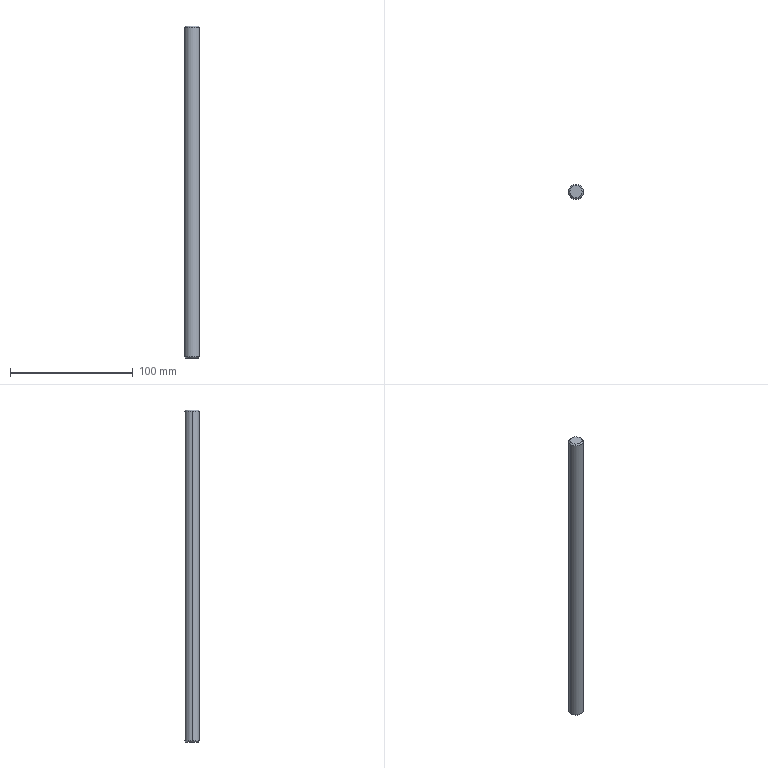Part | STEP file | BPSP-11-11 12Chrome Rod_Default | 1 solid | 12 faces | box 12 x 12 x 270 mm | volume 30254 mm3 | cone 6 | cylinder 4 | plane 2 | commonest cylinder face diameters 4.2 x2 12 x2
STEP:
#1=CARTESIAN_POINT('',(0.,0.,0.));
#2=DIRECTION('',(0.,0.,1.));
#3=DIRECTION('',(1.,0.,0.));
#4=AXIS2_PLACEMENT_3D('',#1,#2,#3);
#5=CARTESIAN_POINT('',(-2.1,0.,17.4));
#6=VERTEX_POINT('',#5);
#7=CARTESIAN_POINT('',(-2.1,0.,0.));
#8=VERTEX_POINT('',#7);
#9=CARTESIAN_POINT('',(-2.1,0.,0.));
#10=DIRECTION('',(0.,0.,-1.));
#11=VECTOR('',#10,1.);
#12=LINE('',#9,#11);
#13=CARTESIAN_POINT('',(0.,0.,0.));
#14=DIRECTION('',(0.,0.,-1.));
#15=DIRECTION('',(-1.,0.,0.));
#16=AXIS2_PLACEMENT_3D('',#13,#14,#15);
#17=CYLINDRICAL_SURFACE('',#16,2.1);
#18=CARTESIAN_POINT('',(6.283,0.));
#19=DIRECTION('',(0.,1.));
#20=VECTOR('',#19,1.);
#21=LINE('',#18,#20);
#22=(GEOMETRIC_REPRESENTATION_CONTEXT(2)PARAMETRIC_REPRESENTATION_CONTEXT()REPRESENTATION_CONTEXT('',''));
#23=DEFINITIONAL_REPRESENTATION('',(#21),#22);
#24=PCURVE('',#17,#23);
#25=CARTESIAN_POINT('',(0.,0.,0.));
#26=DIRECTION('',(0.,0.,-1.));
#27=DIRECTION('',(-1.,0.,0.));
#28=AXIS2_PLACEMENT_3D('',#25,#26,#27);
#29=CYLINDRICAL_SURFACE('',#28,2.1);
#30=CARTESIAN_POINT('',(0.,0.));
#31=DIRECTION('',(0.,1.));
#32=VECTOR('',#31,1.);
#33=LINE('',#30,#32);
#34=(GEOMETRIC_REPRESENTATION_CONTEXT(2)PARAMETRIC_REPRESENTATION_CONTEXT()REPRESENTATION_CONTEXT('',''));
#35=DEFINITIONAL_REPRESENTATION('',(#33),#34);
#36=PCURVE('',#29,#35);
#37=SURFACE_CURVE('',#12,(#24,#36),.PCURVE_S1.);
#38=EDGE_CURVE('',#6,#8,#37,.T.);
#39=ORIENTED_EDGE('',*,*,#38,.T.);
#40=CARTESIAN_POINT('',(2.1,0.,0.));
#41=VERTEX_POINT('',#40);
#42=CARTESIAN_POINT('',(0.,0.,0.));
#43=DIRECTION('',(0.,0.,-1.));
#44=DIRECTION('',(-1.,0.,0.));
#45=AXIS2_PLACEMENT_3D('',#42,#43,#44);
#46=CIRCLE('',#45,2.1);
#47=CARTESIAN_POINT('',(0.,0.));
#48=DIRECTION('',(1.,0.));
#49=VECTOR('',#48,1.);
#50=LINE('',#47,#49);
#51=(GEOMETRIC_REPRESENTATION_CONTEXT(2)PARAMETRIC_REPRESENTATION_CONTEXT()REPRESENTATION_CONTEXT('',''));
#52=DEFINITIONAL_REPRESENTATION('',(#50),#51);
#53=PCURVE('',#17,#52);
#54=CARTESIAN_POINT('',(0.,0.,0.));
#55=DIRECTION('',(0.,0.,1.));
#56=DIRECTION('',(1.,0.,0.));
#57=AXIS2_PLACEMENT_3D('',#54,#55,#56);
#58=PLANE('',#57);
#59=CARTESIAN_POINT('',(-2.1,0.));
#60=CARTESIAN_POINT('',(-2.1,3.637));
#61=CARTESIAN_POINT('',(1.05,1.819));
#62=CARTESIAN_POINT('',(4.2,0.));
#63=CARTESIAN_POINT('',(1.05,-1.819));
#64=CARTESIAN_POINT('',(-2.1,-3.637));
#65=CARTESIAN_POINT('',(-2.1,0.));
#66=(BOUNDED_CURVE()B_SPLINE_CURVE(2,(#59,#60,#61,#62,#63,#64,#65),.UNSPECIFIED.,.T.,.F.)B_SPLINE_CURVE_WITH_KNOTS((1,2,2,2,2,1),(-2.094,0.,2.094,4.189,6.283,8.378),.UNSPECIFIED.)CURVE()GEOMETRIC_REPRESENTATION_ITEM()RATIONAL_B_SPLINE_CURVE((1.,0.5,1.,0.5,1.,0.5,1.))REPRESENTATION_ITEM(''));
#67=(GEOMETRIC_REPRESENTATION_CONTEXT(2)PARAMETRIC_REPRESENTATION_CONTEXT()REPRESENTATION_CONTEXT('',''));
#68=DEFINITIONAL_REPRESENTATION('',(#66),#67);
#69=PCURVE('',#58,#68);
#70=SURFACE_CURVE('',#46,(#53,#69),.PCURVE_S1.);
#71=EDGE_CURVE('',#41,#8,#70,.T.);
#72=ORIENTED_EDGE('',*,*,#71,.F.);
#73=CARTESIAN_POINT('',(2.1,0.,17.4));
#74=VERTEX_POINT('',#73);
#75=CARTESIAN_POINT('',(2.1,0.,0.));
#76=DIRECTION('',(0.,0.,-1.));
#77=VECTOR('',#76,1.);
#78=LINE('',#75,#77);
#79=CARTESIAN_POINT('',(3.142,0.));
#80=DIRECTION('',(0.,1.));
#81=VECTOR('',#80,1.);
#82=LINE('',#79,#81);
#83=(GEOMETRIC_REPRESENTATION_CONTEXT(2)PARAMETRIC_REPRESENTATION_CONTEXT()REPRESENTATION_CONTEXT('',''));
#84=DEFINITIONAL_REPRESENTATION('',(#82),#83);
#85=PCURVE('',#17,#84);
#86=CARTESIAN_POINT('',(3.142,0.));
#87=DIRECTION('',(0.,1.));
#88=VECTOR('',#87,1.);
#89=LINE('',#86,#88);
#90=(GEOMETRIC_REPRESENTATION_CONTEXT(2)PARAMETRIC_REPRESENTATION_CONTEXT()REPRESENTATION_CONTEXT('',''));
#91=DEFINITIONAL_REPRESENTATION('',(#89),#90);
#92=PCURVE('',#29,#91);
#93=SURFACE_CURVE('',#78,(#85,#92),.PCURVE_S1.);
#94=EDGE_CURVE('',#74,#41,#93,.T.);
#95=ORIENTED_EDGE('',*,*,#94,.F.);
#96=CARTESIAN_POINT('',(0.,0.,17.4));
#97=DIRECTION('',(0.,0.,-1.));
#98=DIRECTION('',(-1.,0.,0.));
#99=AXIS2_PLACEMENT_3D('',#96,#97,#98);
#100=CIRCLE('',#99,2.1);
#101=CARTESIAN_POINT('',(0.,-17.4));
#102=DIRECTION('',(1.,0.));
#103=VECTOR('',#102,1.);
#104=LINE('',#101,#103);
#105=(GEOMETRIC_REPRESENTATION_CONTEXT(2)PARAMETRIC_REPRESENTATION_CONTEXT()REPRESENTATION_CONTEXT('',''));
#106=DEFINITIONAL_REPRESENTATION('',(#104),#105);
#107=PCURVE('',#17,#106);
#108=CARTESIAN_POINT('',(0.,0.,17.4));
#109=DIRECTION('',(0.,0.,-1.));
#110=DIRECTION('',(-1.,0.,0.));
#111=AXIS2_PLACEMENT_3D('',#108,#109,#110);
#112=CONICAL_SURFACE('',#111,2.1,1.03);
#113=CARTESIAN_POINT('',(0.,0.));
#114=DIRECTION('',(1.,0.));
#115=VECTOR('',#114,1.);
#116=LINE('',#113,#115);
#117=(GEOMETRIC_REPRESENTATION_CONTEXT(2)PARAMETRIC_REPRESENTATION_CONTEXT()REPRESENTATION_CONTEXT('',''));
#118=DEFINITIONAL_REPRESENTATION('',(#116),#117);
#119=PCURVE('',#112,#118);
#120=SURFACE_CURVE('',#100,(#107,#119),.PCURVE_S1.);
#121=EDGE_CURVE('',#74,#6,#120,.T.);
#122=ORIENTED_EDGE('',*,*,#121,.T.);
#123=EDGE_LOOP('',(#39,#72,#95,#122));
#124=FACE_BOUND('',#123,.F.);
#125=ADVANCED_FACE('',(#124),#17,.F.);
#126=ORIENTED_EDGE('',*,*,#121,.F.);
#127=CARTESIAN_POINT('',(0.,0.,18.662));
#128=VERTEX_POINT('',#127);
#129=CARTESIAN_POINT('',(2.1,0.,17.4));
#130=DIRECTION('',(0.8572,0.,-0.515));
#131=VECTOR('',#130,1.);
#132=LINE('',#129,#131);
#133=CARTESIAN_POINT('',(3.142,0.));
#134=DIRECTION('',(0.,1.));
#135=VECTOR('',#134,1.);
#136=LINE('',#133,#135);
#137=(GEOMETRIC_REPRESENTATION_CONTEXT(2)PARAMETRIC_REPRESENTATION_CONTEXT()REPRESENTATION_CONTEXT('',''));
#138=DEFINITIONAL_REPRESENTATION('',(#136),#137);
#139=PCURVE('',#112,#138);
#140=CARTESIAN_POINT('',(0.,0.,17.4));
#141=DIRECTION('',(0.,0.,-1.));
#142=DIRECTION('',(-1.,0.,0.));
#143=AXIS2_PLACEMENT_3D('',#140,#141,#142);
#144=CONICAL_SURFACE('',#143,2.1,1.03);
#145=CARTESIAN_POINT('',(3.142,0.));
#146=DIRECTION('',(0.,1.));
#147=VECTOR('',#146,1.);
#148=LINE('',#145,#147);
#149=(GEOMETRIC_REPRESENTATION_CONTEXT(2)PARAMETRIC_REPRESENTATION_CONTEXT()REPRESENTATION_CONTEXT('',''));
#150=DEFINITIONAL_REPRESENTATION('',(#148),#149);
#151=PCURVE('',#144,#150);
#152=SURFACE_CURVE('',#132,(#139,#151),.PCURVE_S1.);
#153=EDGE_CURVE('',#128,#74,#152,.T.);
#154=ORIENTED_EDGE('',*,*,#153,.F.);
#155=CARTESIAN_POINT('',(-2.1,0.,17.4));
#156=DIRECTION('',(-0.8572,0.,-0.515));
#157=VECTOR('',#156,1.);
#158=LINE('',#155,#157);
#159=CARTESIAN_POINT('',(6.283,0.));
#160=DIRECTION('',(0.,1.));
#161=VECTOR('',#160,1.);
#162=LINE('',#159,#161);
#163=(GEOMETRIC_REPRESENTATION_CONTEXT(2)PARAMETRIC_REPRESENTATION_CONTEXT()REPRESENTATION_CONTEXT('',''));
#164=DEFINITIONAL_REPRESENTATION('',(#162),#163);
#165=PCURVE('',#112,#164);
#166=CARTESIAN_POINT('',(0.,0.));
#167=DIRECTION('',(0.,1.));
#168=VECTOR('',#167,1.);
#169=LINE('',#166,#168);
#170=(GEOMETRIC_REPRESENTATION_CONTEXT(2)PARAMETRIC_REPRESENTATION_CONTEXT()REPRESENTATION_CONTEXT('',''));
#171=DEFINITIONAL_REPRESENTATION('',(#169),#170);
#172=PCURVE('',#144,#171);
#173=SURFACE_CURVE('',#158,(#165,#172),.PCURVE_S1.);
#174=EDGE_CURVE('',#128,#6,#173,.T.);
#175=ORIENTED_EDGE('',*,*,#174,.T.);
#176=EDGE_LOOP('',(#126,#154,#175));
#177=FACE_BOUND('',#176,.F.);
#178=ADVANCED_FACE('',(#177),#112,.F.);
#179=CARTESIAN_POINT('',(5.,0.,270.));
#180=VERTEX_POINT('',#179);
#181=CARTESIAN_POINT('',(-5.,0.,270.));
#182=VERTEX_POINT('',#181);
#183=CARTESIAN_POINT('',(0.,0.,270.));
#184=DIRECTION('',(0.,0.,1.));
#185=DIRECTION('',(1.,0.,0.));
#186=AXIS2_PLACEMENT_3D('',#183,#184,#185);
#187=CIRCLE('',#186,5.);
#188=CARTESIAN_POINT('',(0.,0.,270.));
#189=DIRECTION('',(0.,0.,-1.));
#190=DIRECTION('',(-1.,0.,0.));
#191=AXIS2_PLACEMENT_3D('',#188,#189,#190);
#192=CONICAL_SURFACE('',#191,5.,0.7854);
#193=CARTESIAN_POINT('',(3.142,0.));
#194=DIRECTION('',(-1.,0.));
#195=VECTOR('',#194,1.);
#196=LINE('',#193,#195);
#197=(GEOMETRIC_REPRESENTATION_CONTEXT(2)PARAMETRIC_REPRESENTATION_CONTEXT()REPRESENTATION_CONTEXT('',''));
#198=DEFINITIONAL_REPRESENTATION('',(#196),#197);
#199=PCURVE('',#192,#198);
#200=CARTESIAN_POINT('',(0.,0.,270.));
#201=DIRECTION('',(0.,0.,1.));
#202=DIRECTION('',(1.,0.,0.));
#203=AXIS2_PLACEMENT_3D('',#200,#201,#202);
#204=PLANE('',#203);
#205=CARTESIAN_POINT('',(0.,0.));
#206=DIRECTION('',(1.,0.));
#207=AXIS2_PLACEMENT_2D('',#205,#206);
#208=CIRCLE('',#207,5.);
#209=(GEOMETRIC_REPRESENTATION_CONTEXT(2)PARAMETRIC_REPRESENTATION_CONTEXT()REPRESENTATION_CONTEXT('',''));
#210=DEFINITIONAL_REPRESENTATION('',(#208),#209);
#211=PCURVE('',#204,#210);
#212=SURFACE_CURVE('',#187,(#199,#211),.PCURVE_S1.);
#213=EDGE_CURVE('',#180,#182,#212,.T.);
#214=ORIENTED_EDGE('',*,*,#213,.F.);
#215=CARTESIAN_POINT('',(6.,0.,269.));
#216=VERTEX_POINT('',#215);
#217=CARTESIAN_POINT('',(5.,0.,270.));
#218=DIRECTION('',(0.7071,0.,-0.7071));
#219=VECTOR('',#218,1.);
#220=LINE('',#217,#219);
#221=CARTESIAN_POINT('',(3.142,0.));
#222=DIRECTION('',(0.,1.));
#223=VECTOR('',#222,1.);
#224=LINE('',#221,#223);
#225=(GEOMETRIC_REPRESENTATION_CONTEXT(2)PARAMETRIC_REPRESENTATION_CONTEXT()REPRESENTATION_CONTEXT('',''));
#226=DEFINITIONAL_REPRESENTATION('',(#224),#225);
#227=PCURVE('',#192,#226);
#228=CARTESIAN_POINT('',(0.,0.,270.));
#229=DIRECTION('',(0.,0.,-1.));
#230=DIRECTION('',(-1.,0.,0.));
#231=AXIS2_PLACEMENT_3D('',#228,#229,#230);
#232=CONICAL_SURFACE('',#231,5.,0.7854);
#233=CARTESIAN_POINT('',(3.142,0.));
#234=DIRECTION('',(0.,1.));
#235=VECTOR('',#234,1.);
#236=LINE('',#233,#235);
#237=(GEOMETRIC_REPRESENTATION_CONTEXT(2)PARAMETRIC_REPRESENTATION_CONTEXT()REPRESENTATION_CONTEXT('',''));
#238=DEFINITIONAL_REPRESENTATION('',(#236),#237);
#239=PCURVE('',#232,#238);
#240=SURFACE_CURVE('',#220,(#227,#239),.PCURVE_S1.);
#241=EDGE_CURVE('',#180,#216,#240,.T.);
#242=ORIENTED_EDGE('',*,*,#241,.T.);
#243=CARTESIAN_POINT('',(-6.,0.,269.));
#244=VERTEX_POINT('',#243);
#245=CARTESIAN_POINT('',(0.,0.,269.));
#246=DIRECTION('',(0.,0.,-1.));
#247=DIRECTION('',(1.,0.,0.));
#248=AXIS2_PLACEMENT_3D('',#245,#246,#247);
#249=CIRCLE('',#248,6.);
#250=CARTESIAN_POINT('',(-3.142,1.));
#251=DIRECTION('',(1.,0.));
#252=VECTOR('',#251,1.);
#253=LINE('',#250,#252);
#254=(GEOMETRIC_REPRESENTATION_CONTEXT(2)PARAMETRIC_REPRESENTATION_CONTEXT()REPRESENTATION_CONTEXT('',''));
#255=DEFINITIONAL_REPRESENTATION('',(#253),#254);
#256=PCURVE('',#192,#255);
#257=CARTESIAN_POINT('',(0.,0.,270.));
#258=DIRECTION('',(0.,0.,-1.));
#259=DIRECTION('',(-1.,0.,0.));
#260=AXIS2_PLACEMENT_3D('',#257,#258,#259);
#261=CYLINDRICAL_SURFACE('',#260,6.);
#262=CARTESIAN_POINT('',(-3.142,1.));
#263=DIRECTION('',(1.,0.));
#264=VECTOR('',#263,1.);
#265=LINE('',#262,#264);
#266=(GEOMETRIC_REPRESENTATION_CONTEXT(2)PARAMETRIC_REPRESENTATION_CONTEXT()REPRESENTATION_CONTEXT('',''));
#267=DEFINITIONAL_REPRESENTATION('',(#265),#266);
#268=PCURVE('',#261,#267);
#269=SURFACE_CURVE('',#249,(#256,#268),.PCURVE_S1.);
#270=EDGE_CURVE('',#244,#216,#269,.T.);
#271=ORIENTED_EDGE('',*,*,#270,.F.);
#272=CARTESIAN_POINT('',(-5.,0.,270.));
#273=DIRECTION('',(-0.7071,0.,-0.7071));
#274=VECTOR('',#273,1.);
#275=LINE('',#272,#274);
#276=CARTESIAN_POINT('',(0.,0.));
#277=DIRECTION('',(0.,1.));
#278=VECTOR('',#277,1.);
#279=LINE('',#276,#278);
#280=(GEOMETRIC_REPRESENTATION_CONTEXT(2)PARAMETRIC_REPRESENTATION_CONTEXT()REPRESENTATION_CONTEXT('',''));
#281=DEFINITIONAL_REPRESENTATION('',(#279),#280);
#282=PCURVE('',#192,#281);
#283=CARTESIAN_POINT('',(6.283,0.));
#284=DIRECTION('',(0.,1.));
#285=VECTOR('',#284,1.);
#286=LINE('',#283,#285);
#287=(GEOMETRIC_REPRESENTATION_CONTEXT(2)PARAMETRIC_REPRESENTATION_CONTEXT()REPRESENTATION_CONTEXT('',''));
#288=DEFINITIONAL_REPRESENTATION('',(#286),#287);
#289=PCURVE('',#232,#288);
#290=SURFACE_CURVE('',#275,(#282,#289),.PCURVE_S1.);
#291=EDGE_CURVE('',#182,#244,#290,.T.);
#292=ORIENTED_EDGE('',*,*,#291,.F.);
#293=EDGE_LOOP('',(#214,#242,#271,#292));
#294=FACE_BOUND('',#293,.T.);
#295=ADVANCED_FACE('',(#294),#192,.T.);
#296=CARTESIAN_POINT('',(-5.,0.,0.));
#297=VERTEX_POINT('',#296);
#298=CARTESIAN_POINT('',(5.,0.,0.));
#299=VERTEX_POINT('',#298);
#300=CARTESIAN_POINT('',(0.,0.,0.));
#301=DIRECTION('',(0.,0.,-1.));
#302=DIRECTION('',(1.,0.,0.));
#303=AXIS2_PLACEMENT_3D('',#300,#301,#302);
#304=CIRCLE('',#303,5.);
#305=CARTESIAN_POINT('',(0.,0.,1.));
#306=DIRECTION('',(0.,0.,1.));
#307=DIRECTION('',(1.,0.,0.));
#308=AXIS2_PLACEMENT_3D('',#305,#306,#307);
#309=CONICAL_SURFACE('',#308,6.,0.7854);
#310=CARTESIAN_POINT('',(6.283,-1.));
#311=DIRECTION('',(-1.,0.));
#312=VECTOR('',#311,1.);
#313=LINE('',#310,#312);
#314=(GEOMETRIC_REPRESENTATION_CONTEXT(2)PARAMETRIC_REPRESENTATION_CONTEXT()REPRESENTATION_CONTEXT('',''));
#315=DEFINITIONAL_REPRESENTATION('',(#313),#314);
#316=PCURVE('',#309,#315);
#317=CARTESIAN_POINT('',(5.,0.));
#318=CARTESIAN_POINT('',(5.,-8.66));
#319=CARTESIAN_POINT('',(-2.5,-4.33));
#320=CARTESIAN_POINT('',(-10.,0.));
#321=CARTESIAN_POINT('',(-2.5,4.33));
#322=CARTESIAN_POINT('',(5.,8.66));
#323=CARTESIAN_POINT('',(5.,0.));
#324=(BOUNDED_CURVE()B_SPLINE_CURVE(2,(#317,#318,#319,#320,#321,#322,#323),.UNSPECIFIED.,.T.,.F.)B_SPLINE_CURVE_WITH_KNOTS((1,2,2,2,2,1),(-2.094,0.,2.094,4.189,6.283,8.378),.UNSPECIFIED.)CURVE()GEOMETRIC_REPRESENTATION_ITEM()RATIONAL_B_SPLINE_CURVE((1.,0.5,1.,0.5,1.,0.5,1.))REPRESENTATION_ITEM(''));
#325=(GEOMETRIC_REPRESENTATION_CONTEXT(2)PARAMETRIC_REPRESENTATION_CONTEXT()REPRESENTATION_CONTEXT('',''));
#326=DEFINITIONAL_REPRESENTATION('',(#324),#325);
#327=PCURVE('',#58,#326);
#328=SURFACE_CURVE('',#304,(#316,#327),.PCURVE_S1.);
#329=EDGE_CURVE('',#297,#299,#328,.T.);
#330=ORIENTED_EDGE('',*,*,#329,.F.);
#331=CARTESIAN_POINT('',(-6.,0.,1.));
#332=VERTEX_POINT('',#331);
#333=CARTESIAN_POINT('',(-6.,0.,1.));
#334=DIRECTION('',(-0.7071,0.,0.7071));
#335=VECTOR('',#334,1.);
#336=LINE('',#333,#335);
#337=CARTESIAN_POINT('',(3.142,0.));
#338=DIRECTION('',(0.,1.));
#339=VECTOR('',#338,1.);
#340=LINE('',#337,#339);
#341=(GEOMETRIC_REPRESENTATION_CONTEXT(2)PARAMETRIC_REPRESENTATION_CONTEXT()REPRESENTATION_CONTEXT('',''));
#342=DEFINITIONAL_REPRESENTATION('',(#340),#341);
#343=PCURVE('',#309,#342);
#344=CARTESIAN_POINT('',(0.,0.,1.));
#345=DIRECTION('',(0.,0.,1.));
#346=DIRECTION('',(1.,0.,0.));
#347=AXIS2_PLACEMENT_3D('',#344,#345,#346);
#348=CONICAL_SURFACE('',#347,6.,0.7854);
#349=CARTESIAN_POINT('',(3.142,0.));
#350=DIRECTION('',(0.,1.));
#351=VECTOR('',#350,1.);
#352=LINE('',#349,#351);
#353=(GEOMETRIC_REPRESENTATION_CONTEXT(2)PARAMETRIC_REPRESENTATION_CONTEXT()REPRESENTATION_CONTEXT('',''));
#354=DEFINITIONAL_REPRESENTATION('',(#352),#353);
#355=PCURVE('',#348,#354);
#356=SURFACE_CURVE('',#336,(#343,#355),.PCURVE_S1.);
#357=EDGE_CURVE('',#297,#332,#356,.T.);
#358=ORIENTED_EDGE('',*,*,#357,.T.);
#359=CARTESIAN_POINT('',(6.,0.,1.));
#360=VERTEX_POINT('',#359);
#361=CARTESIAN_POINT('',(0.,0.,1.));
#362=DIRECTION('',(0.,0.,1.));
#363=DIRECTION('',(1.,0.,0.));
#364=AXIS2_PLACEMENT_3D('',#361,#362,#363);
#365=CIRCLE('',#364,6.);
#366=CARTESIAN_POINT('',(0.,0.));
#367=DIRECTION('',(1.,0.));
#368=VECTOR('',#367,1.);
#369=LINE('',#366,#368);
#370=(GEOMETRIC_REPRESENTATION_CONTEXT(2)PARAMETRIC_REPRESENTATION_CONTEXT()REPRESENTATION_CONTEXT('',''));
#371=DEFINITIONAL_REPRESENTATION('',(#369),#370);
#372=PCURVE('',#309,#371);
#373=CARTESIAN_POINT('',(3.142,269.));
#374=DIRECTION('',(-1.,0.));
#375=VECTOR('',#374,1.);
#376=LINE('',#373,#375);
#377=(GEOMETRIC_REPRESENTATION_CONTEXT(2)PARAMETRIC_REPRESENTATION_CONTEXT()REPRESENTATION_CONTEXT('',''));
#378=DEFINITIONAL_REPRESENTATION('',(#376),#377);
#379=PCURVE('',#261,#378);
#380=SURFACE_CURVE('',#365,(#372,#379),.PCURVE_S1.);
#381=EDGE_CURVE('',#360,#332,#380,.T.);
#382=ORIENTED_EDGE('',*,*,#381,.F.);
#383=CARTESIAN_POINT('',(6.,0.,1.));
#384=DIRECTION('',(0.7071,0.,0.7071));
#385=VECTOR('',#384,1.);
#386=LINE('',#383,#385);
#387=CARTESIAN_POINT('',(0.,0.));
#388=DIRECTION('',(0.,1.));
#389=VECTOR('',#388,1.);
#390=LINE('',#387,#389);
#391=(GEOMETRIC_REPRESENTATION_CONTEXT(2)PARAMETRIC_REPRESENTATION_CONTEXT()REPRESENTATION_CONTEXT('',''));
#392=DEFINITIONAL_REPRESENTATION('',(#390),#391);
#393=PCURVE('',#309,#392);
#394=CARTESIAN_POINT('',(6.283,0.));
#395=DIRECTION('',(0.,1.));
#396=VECTOR('',#395,1.);
#397=LINE('',#394,#396);
#398=(GEOMETRIC_REPRESENTATION_CONTEXT(2)PARAMETRIC_REPRESENTATION_CONTEXT()REPRESENTATION_CONTEXT('',''));
#399=DEFINITIONAL_REPRESENTATION('',(#397),#398);
#400=PCURVE('',#348,#399);
#401=SURFACE_CURVE('',#386,(#393,#400),.PCURVE_S1.);
#402=EDGE_CURVE('',#299,#360,#401,.T.);
#403=ORIENTED_EDGE('',*,*,#402,.F.);
#404=EDGE_LOOP('',(#330,#358,#382,#403));
#405=FACE_BOUND('',#404,.T.);
#406=ADVANCED_FACE('',(#405),#309,.T.);
#407=ORIENTED_EDGE('',*,*,#270,.T.);
#408=CARTESIAN_POINT('',(6.,0.,270.));
#409=DIRECTION('',(0.,0.,-1.));
#410=VECTOR('',#409,1.);
#411=LINE('',#408,#410);
#412=CARTESIAN_POINT('',(3.142,0.));
#413=DIRECTION('',(0.,1.));
#414=VECTOR('',#413,1.);
#415=LINE('',#412,#414);
#416=(GEOMETRIC_REPRESENTATION_CONTEXT(2)PARAMETRIC_REPRESENTATION_CONTEXT()REPRESENTATION_CONTEXT('',''));
#417=DEFINITIONAL_REPRESENTATION('',(#415),#416);
#418=PCURVE('',#261,#417);
#419=CARTESIAN_POINT('',(0.,0.,270.));
#420=DIRECTION('',(0.,0.,-1.));
#421=DIRECTION('',(-1.,0.,0.));
#422=AXIS2_PLACEMENT_3D('',#419,#420,#421);
#423=CYLINDRICAL_SURFACE('',#422,6.);
#424=CARTESIAN_POINT('',(3.142,0.));
#425=DIRECTION('',(0.,1.));
#426=VECTOR('',#425,1.);
#427=LINE('',#424,#426);
#428=(GEOMETRIC_REPRESENTATION_CONTEXT(2)PARAMETRIC_REPRESENTATION_CONTEXT()REPRESENTATION_CONTEXT('',''));
#429=DEFINITIONAL_REPRESENTATION('',(#427),#428);
#430=PCURVE('',#423,#429);
#431=SURFACE_CURVE('',#411,(#418,#430),.PCURVE_S1.);
#432=EDGE_CURVE('',#216,#360,#431,.T.);
#433=ORIENTED_EDGE('',*,*,#432,.T.);
#434=ORIENTED_EDGE('',*,*,#381,.T.);
#435=CARTESIAN_POINT('',(-6.,0.,270.));
#436=DIRECTION('',(0.,0.,-1.));
#437=VECTOR('',#436,1.);
#438=LINE('',#435,#437);
#439=CARTESIAN_POINT('',(0.,0.));
#440=DIRECTION('',(0.,1.));
#441=VECTOR('',#440,1.);
#442=LINE('',#439,#441);
#443=(GEOMETRIC_REPRESENTATION_CONTEXT(2)PARAMETRIC_REPRESENTATION_CONTEXT()REPRESENTATION_CONTEXT('',''));
#444=DEFINITIONAL_REPRESENTATION('',(#442),#443);
#445=PCURVE('',#261,#444);
#446=CARTESIAN_POINT('',(6.283,0.));
#447=DIRECTION('',(0.,1.));
#448=VECTOR('',#447,1.);
#449=LINE('',#446,#448);
#450=(GEOMETRIC_REPRESENTATION_CONTEXT(2)PARAMETRIC_REPRESENTATION_CONTEXT()REPRESENTATION_CONTEXT('',''));
#451=DEFINITIONAL_REPRESENTATION('',(#449),#450);
#452=PCURVE('',#423,#451);
#453=SURFACE_CURVE('',#438,(#445,#452),.PCURVE_S1.);
#454=EDGE_CURVE('',#244,#332,#453,.T.);
#455=ORIENTED_EDGE('',*,*,#454,.F.);
#456=EDGE_LOOP('',(#407,#433,#434,#455));
#457=FACE_BOUND('',#456,.T.);
#458=ADVANCED_FACE('',(#457),#261,.T.);
#459=ORIENTED_EDGE('',*,*,#432,.F.);
#460=CARTESIAN_POINT('',(0.,0.,269.));
#461=DIRECTION('',(0.,0.,-1.));
#462=DIRECTION('',(1.,0.,0.));
#463=AXIS2_PLACEMENT_3D('',#460,#461,#462);
#464=CIRCLE('',#463,6.);
#465=CARTESIAN_POINT('',(3.142,1.));
#466=DIRECTION('',(1.,0.));
#467=VECTOR('',#466,1.);
#468=LINE('',#465,#467);
#469=(GEOMETRIC_REPRESENTATION_CONTEXT(2)PARAMETRIC_REPRESENTATION_CONTEXT()REPRESENTATION_CONTEXT('',''));
#470=DEFINITIONAL_REPRESENTATION('',(#468),#469);
#471=PCURVE('',#423,#470);
#472=CARTESIAN_POINT('',(3.142,1.));
#473=DIRECTION('',(1.,0.));
#474=VECTOR('',#473,1.);
#475=LINE('',#472,#474);
#476=(GEOMETRIC_REPRESENTATION_CONTEXT(2)PARAMETRIC_REPRESENTATION_CONTEXT()REPRESENTATION_CONTEXT('',''));
#477=DEFINITIONAL_REPRESENTATION('',(#475),#476);
#478=PCURVE('',#232,#477);
#479=SURFACE_CURVE('',#464,(#471,#478),.PCURVE_S1.);
#480=EDGE_CURVE('',#216,#244,#479,.T.);
#481=ORIENTED_EDGE('',*,*,#480,.T.);
#482=ORIENTED_EDGE('',*,*,#454,.T.);
#483=CARTESIAN_POINT('',(0.,0.,1.));
#484=DIRECTION('',(0.,0.,1.));
#485=DIRECTION('',(1.,0.,0.));
#486=AXIS2_PLACEMENT_3D('',#483,#484,#485);
#487=CIRCLE('',#486,6.);
#488=CARTESIAN_POINT('',(9.425,269.));
#489=DIRECTION('',(-1.,0.));
#490=VECTOR('',#489,1.);
#491=LINE('',#488,#490);
#492=(GEOMETRIC_REPRESENTATION_CONTEXT(2)PARAMETRIC_REPRESENTATION_CONTEXT()REPRESENTATION_CONTEXT('',''));
#493=DEFINITIONAL_REPRESENTATION('',(#491),#492);
#494=PCURVE('',#423,#493);
#495=CARTESIAN_POINT('',(0.,0.));
#496=DIRECTION('',(1.,0.));
#497=VECTOR('',#496,1.);
#498=LINE('',#495,#497);
#499=(GEOMETRIC_REPRESENTATION_CONTEXT(2)PARAMETRIC_REPRESENTATION_CONTEXT()REPRESENTATION_CONTEXT('',''));
#500=DEFINITIONAL_REPRESENTATION('',(#498),#499);
#501=PCURVE('',#348,#500);
#502=SURFACE_CURVE('',#487,(#494,#501),.PCURVE_S1.);
#503=EDGE_CURVE('',#332,#360,#502,.T.);
#504=ORIENTED_EDGE('',*,*,#503,.T.);
#505=EDGE_LOOP('',(#459,#481,#482,#504));
#506=FACE_BOUND('',#505,.T.);
#507=ADVANCED_FACE('',(#506),#423,.T.);
#508=CARTESIAN_POINT('',(0.,0.,270.));
#509=DIRECTION('',(0.,0.,1.));
#510=DIRECTION('',(1.,0.,0.));
#511=AXIS2_PLACEMENT_3D('',#508,#509,#510);
#512=CIRCLE('',#511,5.);
#513=CARTESIAN_POINT('',(0.,0.));
#514=DIRECTION('',(1.,0.));
#515=AXIS2_PLACEMENT_2D('',#513,#514);
#516=CIRCLE('',#515,5.);
#517=(GEOMETRIC_REPRESENTATION_CONTEXT(2)PARAMETRIC_REPRESENTATION_CONTEXT()REPRESENTATION_CONTEXT('',''));
#518=DEFINITIONAL_REPRESENTATION('',(#516),#517);
#519=PCURVE('',#204,#518);
#520=CARTESIAN_POINT('',(9.425,0.));
#521=DIRECTION('',(-1.,0.));
#522=VECTOR('',#521,1.);
#523=LINE('',#520,#522);
#524=(GEOMETRIC_REPRESENTATION_CONTEXT(2)PARAMETRIC_REPRESENTATION_CONTEXT()REPRESENTATION_CONTEXT('',''));
#525=DEFINITIONAL_REPRESENTATION('',(#523),#524);
#526=PCURVE('',#232,#525);
#527=SURFACE_CURVE('',#512,(#519,#526),.PCURVE_S1.);
#528=EDGE_CURVE('',#182,#180,#527,.T.);
#529=ORIENTED_EDGE('',*,*,#528,.T.);
#530=ORIENTED_EDGE('',*,*,#213,.T.);
#531=EDGE_LOOP('',(#529,#530));
#532=FACE_BOUND('',#531,.T.);
#533=ADVANCED_FACE('',(#532),#204,.T.);
#534=CARTESIAN_POINT('',(0.,0.,0.));
#535=DIRECTION('',(0.,0.,-1.));
#536=DIRECTION('',(-1.,0.,0.));
#537=AXIS2_PLACEMENT_3D('',#534,#535,#536);
#538=CIRCLE('',#537,2.1);
#539=CARTESIAN_POINT('',(-2.1,0.));
#540=CARTESIAN_POINT('',(-2.1,3.637));
#541=CARTESIAN_POINT('',(1.05,1.819));
#542=CARTESIAN_POINT('',(4.2,0.));
#543=CARTESIAN_POINT('',(1.05,-1.819));
#544=CARTESIAN_POINT('',(-2.1,-3.637));
#545=CARTESIAN_POINT('',(-2.1,0.));
#546=(BOUNDED_CURVE()B_SPLINE_CURVE(2,(#539,#540,#541,#542,#543,#544,#545),.UNSPECIFIED.,.T.,.F.)B_SPLINE_CURVE_WITH_KNOTS((1,2,2,2,2,1),(-2.094,0.,2.094,4.189,6.283,8.378),.UNSPECIFIED.)CURVE()GEOMETRIC_REPRESENTATION_ITEM()RATIONAL_B_SPLINE_CURVE((1.,0.5,1.,0.5,1.,0.5,1.))REPRESENTATION_ITEM(''));
#547=(GEOMETRIC_REPRESENTATION_CONTEXT(2)PARAMETRIC_REPRESENTATION_CONTEXT()REPRESENTATION_CONTEXT('',''));
#548=DEFINITIONAL_REPRESENTATION('',(#546),#547);
#549=PCURVE('',#58,#548);
#550=CARTESIAN_POINT('',(0.,0.));
#551=DIRECTION('',(1.,0.));
#552=VECTOR('',#551,1.);
#553=LINE('',#550,#552);
#554=(GEOMETRIC_REPRESENTATION_CONTEXT(2)PARAMETRIC_REPRESENTATION_CONTEXT()REPRESENTATION_CONTEXT('',''));
#555=DEFINITIONAL_REPRESENTATION('',(#553),#554);
#556=PCURVE('',#29,#555);
#557=SURFACE_CURVE('',#538,(#549,#556),.PCURVE_S1.);
#558=EDGE_CURVE('',#8,#41,#557,.T.);
#559=ORIENTED_EDGE('',*,*,#558,.F.);
#560=ORIENTED_EDGE('',*,*,#71,.F.);
#561=EDGE_LOOP('',(#559,#560));
#562=FACE_BOUND('',#561,.T.);
#563=CARTESIAN_POINT('',(0.,0.,0.));
#564=DIRECTION('',(0.,0.,-1.));
#565=DIRECTION('',(1.,0.,0.));
#566=AXIS2_PLACEMENT_3D('',#563,#564,#565);
#567=CIRCLE('',#566,5.);
#568=CARTESIAN_POINT('',(5.,0.));
#569=CARTESIAN_POINT('',(5.,-8.66));
#570=CARTESIAN_POINT('',(-2.5,-4.33));
#571=CARTESIAN_POINT('',(-10.,0.));
#572=CARTESIAN_POINT('',(-2.5,4.33));
#573=CARTESIAN_POINT('',(5.,8.66));
#574=CARTESIAN_POINT('',(5.,0.));
#575=(BOUNDED_CURVE()B_SPLINE_CURVE(2,(#568,#569,#570,#571,#572,#573,#574),.UNSPECIFIED.,.T.,.F.)B_SPLINE_CURVE_WITH_KNOTS((1,2,2,2,2,1),(-2.094,0.,2.094,4.189,6.283,8.378),.UNSPECIFIED.)CURVE()GEOMETRIC_REPRESENTATION_ITEM()RATIONAL_B_SPLINE_CURVE((1.,0.5,1.,0.5,1.,0.5,1.))REPRESENTATION_ITEM(''));
#576=(GEOMETRIC_REPRESENTATION_CONTEXT(2)PARAMETRIC_REPRESENTATION_CONTEXT()REPRESENTATION_CONTEXT('',''));
#577=DEFINITIONAL_REPRESENTATION('',(#575),#576);
#578=PCURVE('',#58,#577);
#579=CARTESIAN_POINT('',(6.283,-1.));
#580=DIRECTION('',(-1.,0.));
#581=VECTOR('',#580,1.);
#582=LINE('',#579,#581);
#583=(GEOMETRIC_REPRESENTATION_CONTEXT(2)PARAMETRIC_REPRESENTATION_CONTEXT()REPRESENTATION_CONTEXT('',''));
#584=DEFINITIONAL_REPRESENTATION('',(#582),#583);
#585=PCURVE('',#348,#584);
#586=SURFACE_CURVE('',#567,(#578,#585),.PCURVE_S1.);
#587=EDGE_CURVE('',#299,#297,#586,.T.);
#588=ORIENTED_EDGE('',*,*,#587,.T.);
#589=ORIENTED_EDGE('',*,*,#329,.T.);
#590=EDGE_LOOP('',(#588,#589));
#591=FACE_BOUND('',#590,.T.);
#592=ADVANCED_FACE('',(#562,#591),#58,.F.);
#593=ORIENTED_EDGE('',*,*,#357,.F.);
#594=ORIENTED_EDGE('',*,*,#587,.F.);
#595=ORIENTED_EDGE('',*,*,#402,.T.);
#596=ORIENTED_EDGE('',*,*,#503,.F.);
#597=EDGE_LOOP('',(#593,#594,#595,#596));
#598=FACE_BOUND('',#597,.T.);
#599=ADVANCED_FACE('',(#598),#348,.T.);
#600=ORIENTED_EDGE('',*,*,#241,.F.);
#601=ORIENTED_EDGE('',*,*,#528,.F.);
#602=ORIENTED_EDGE('',*,*,#291,.T.);
#603=ORIENTED_EDGE('',*,*,#480,.F.);
#604=EDGE_LOOP('',(#600,#601,#602,#603));
#605=FACE_BOUND('',#604,.T.);
#606=ADVANCED_FACE('',(#605),#232,.T.);
#607=CARTESIAN_POINT('',(0.,0.,17.4));
#608=DIRECTION('',(0.,0.,-1.));
#609=DIRECTION('',(-1.,0.,0.));
#610=AXIS2_PLACEMENT_3D('',#607,#608,#609);
#611=CIRCLE('',#610,2.1);
#612=CARTESIAN_POINT('',(0.,0.));
#613=DIRECTION('',(1.,0.));
#614=VECTOR('',#613,1.);
#615=LINE('',#612,#614);
#616=(GEOMETRIC_REPRESENTATION_CONTEXT(2)PARAMETRIC_REPRESENTATION_CONTEXT()REPRESENTATION_CONTEXT('',''));
#617=DEFINITIONAL_REPRESENTATION('',(#615),#616);
#618=PCURVE('',#144,#617);
#619=CARTESIAN_POINT('',(0.,-17.4));
#620=DIRECTION('',(1.,0.));
#621=VECTOR('',#620,1.);
#622=LINE('',#619,#621);
#623=(GEOMETRIC_REPRESENTATION_CONTEXT(2)PARAMETRIC_REPRESENTATION_CONTEXT()REPRESENTATION_CONTEXT('',''));
#624=DEFINITIONAL_REPRESENTATION('',(#622),#623);
#625=PCURVE('',#29,#624);
#626=SURFACE_CURVE('',#611,(#618,#625),.PCURVE_S1.);
#627=EDGE_CURVE('',#6,#74,#626,.T.);
#628=ORIENTED_EDGE('',*,*,#627,.F.);
#629=ORIENTED_EDGE('',*,*,#174,.F.);
#630=ORIENTED_EDGE('',*,*,#153,.T.);
#631=EDGE_LOOP('',(#628,#629,#630));
#632=FACE_BOUND('',#631,.F.);
#633=ADVANCED_FACE('',(#632),#144,.F.);
#634=ORIENTED_EDGE('',*,*,#558,.F.);
#635=ORIENTED_EDGE('',*,*,#38,.F.);
#636=ORIENTED_EDGE('',*,*,#627,.T.);
#637=ORIENTED_EDGE('',*,*,#94,.T.);
#638=EDGE_LOOP('',(#634,#635,#636,#637));
#639=FACE_BOUND('',#638,.F.);
#640=ADVANCED_FACE('',(#639),#29,.F.);
#641=CLOSED_SHELL('',(#125,#178,#295,#406,#458,#507,#533,#592,#599,#606,#633,#640));
#642=MANIFOLD_SOLID_BREP('',#641);
#643=(LENGTH_UNIT()NAMED_UNIT(*)SI_UNIT(.MILLI.,.METRE.));
#644=UNCERTAINTY_MEASURE_WITH_UNIT(LENGTH_MEASURE(0.0000001),#643,'','');
#645=(NAMED_UNIT(*)PLANE_ANGLE_UNIT()SI_UNIT($,.RADIAN.));
#646=(NAMED_UNIT(*)SI_UNIT($,.STERADIAN.)SOLID_ANGLE_UNIT());
#647=(GEOMETRIC_REPRESENTATION_CONTEXT(3)GLOBAL_UNCERTAINTY_ASSIGNED_CONTEXT((#644))GLOBAL_UNIT_ASSIGNED_CONTEXT((#643,#645,#646))REPRESENTATION_CONTEXT('',''));
#648=ADVANCED_BREP_SHAPE_REPRESENTATION('',(#4,#642),#647);